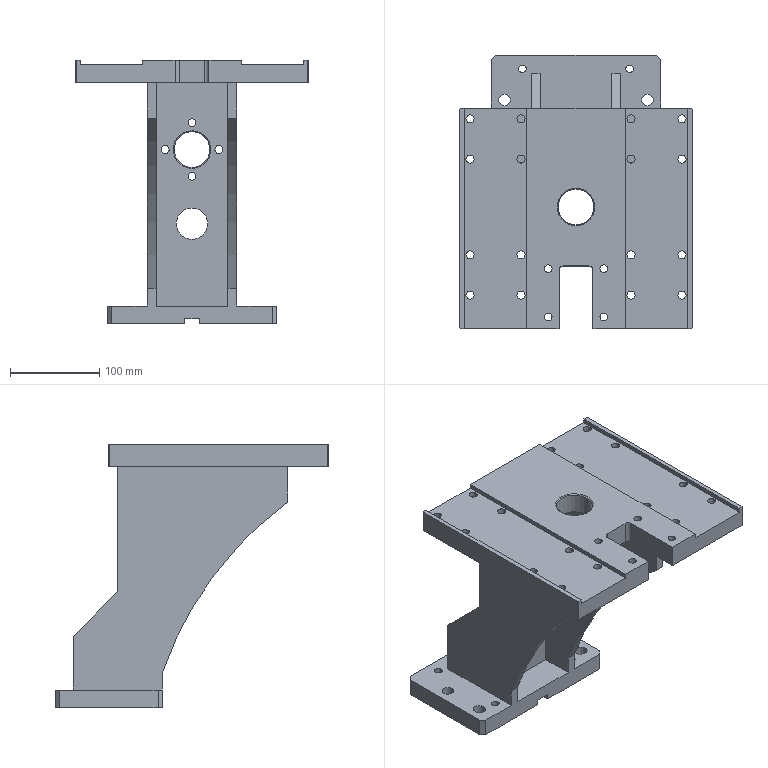Part | STEP file | YCD14007A-08.03.03 Clamping Arm (Right) | 1 solid | 155 faces | box 260 x 306 x 295 mm | volume 2644303 mm3 | cylinder 88 | plane 55 | cone 12 | commonest cylinder face diameters 9 x42 8.5 x16 15 x8 4.2 x4 13 x4 14 x4